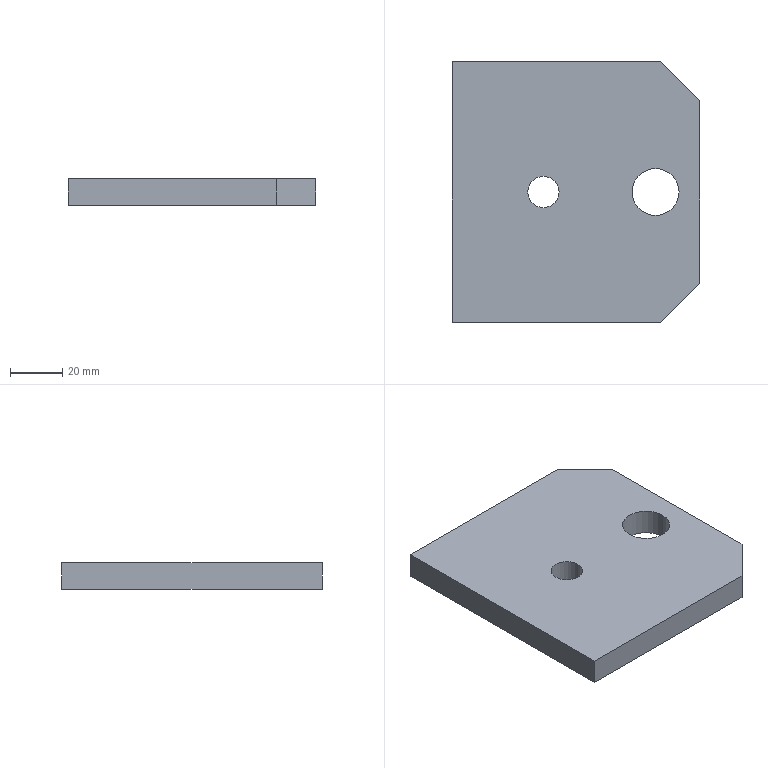Part | SolidWorks | features Extrusion 1 | 1 solid | 12 faces | box 95 x 100 x 10 mm | volume 89074 mm3 | plane 8 | cylinder 4 | commonest cylinder face diameters 12 x2 18 x2
STEP:
#1=CARTESIAN_POINT('',(21.5,0.,10.));
#2=VERTEX_POINT('',#1);
#3=CARTESIAN_POINT('',(39.5,0.,10.));
#4=VERTEX_POINT('',#3);
#5=CARTESIAN_POINT('',(30.5,0.,10.));
#6=DIRECTION('',(0.,0.,1.));
#7=DIRECTION('',(1.,0.,0.));
#8=AXIS2_PLACEMENT_3D('',#5,#6,#7);
#9=CIRCLE('',#8,9.);
#10=EDGE_CURVE('',#2,#4,#9,.T.);
#11=ORIENTED_EDGE('',*,*,#10,.T.);
#12=CARTESIAN_POINT('',(39.5,0.,0.));
#13=VERTEX_POINT('',#12);
#14=CARTESIAN_POINT('',(39.5,0.,10.));
#15=DIRECTION('',(0.,0.,-1.));
#16=VECTOR('',#15,1000.);
#17=LINE('',#14,#16);
#18=EDGE_CURVE('',#4,#13,#17,.T.);
#19=ORIENTED_EDGE('',*,*,#18,.T.);
#20=CARTESIAN_POINT('',(21.5,0.,0.));
#21=VERTEX_POINT('',#20);
#22=CARTESIAN_POINT('',(30.5,0.,0.));
#23=DIRECTION('',(0.,0.,1.));
#24=DIRECTION('',(1.,0.,0.));
#25=AXIS2_PLACEMENT_3D('',#22,#23,#24);
#26=CIRCLE('',#25,9.);
#27=EDGE_CURVE('',#21,#13,#26,.T.);
#28=ORIENTED_EDGE('',*,*,#27,.F.);
#29=CARTESIAN_POINT('',(21.5,0.,10.));
#30=DIRECTION('',(0.,0.,-1.));
#31=VECTOR('',#30,1000.);
#32=LINE('',#29,#31);
#33=EDGE_CURVE('',#2,#21,#32,.T.);
#34=ORIENTED_EDGE('',*,*,#33,.F.);
#35=EDGE_LOOP('',(#11,#19,#28,#34));
#36=FACE_OUTER_BOUND('',#35,.T.);
#37=CARTESIAN_POINT('',(30.5,0.,10.));
#38=DIRECTION('',(0.,0.,-1.));
#39=DIRECTION('',(-1.,0.,0.));
#40=AXIS2_PLACEMENT_3D('',#37,#38,#39);
#41=CYLINDRICAL_SURFACE('',#40,9.);
#42=ADVANCED_FACE('',(#36),#41,.F.);
#43=CARTESIAN_POINT('',(-18.5,0.,10.));
#44=VERTEX_POINT('',#43);
#45=CARTESIAN_POINT('',(-6.5,0.,10.));
#46=VERTEX_POINT('',#45);
#47=CARTESIAN_POINT('',(-12.5,0.,10.));
#48=DIRECTION('',(0.,0.,1.));
#49=DIRECTION('',(1.,0.,0.));
#50=AXIS2_PLACEMENT_3D('',#47,#48,#49);
#51=CIRCLE('',#50,6.);
#52=EDGE_CURVE('',#44,#46,#51,.T.);
#53=ORIENTED_EDGE('',*,*,#52,.T.);
#54=CARTESIAN_POINT('',(-6.5,0.,0.));
#55=VERTEX_POINT('',#54);
#56=CARTESIAN_POINT('',(-6.5,0.,10.));
#57=DIRECTION('',(0.,0.,-1.));
#58=VECTOR('',#57,1000.);
#59=LINE('',#56,#58);
#60=EDGE_CURVE('',#46,#55,#59,.T.);
#61=ORIENTED_EDGE('',*,*,#60,.T.);
#62=CARTESIAN_POINT('',(-18.5,0.,0.));
#63=VERTEX_POINT('',#62);
#64=CARTESIAN_POINT('',(-12.5,0.,0.));
#65=DIRECTION('',(0.,0.,1.));
#66=DIRECTION('',(1.,0.,0.));
#67=AXIS2_PLACEMENT_3D('',#64,#65,#66);
#68=CIRCLE('',#67,6.);
#69=EDGE_CURVE('',#63,#55,#68,.T.);
#70=ORIENTED_EDGE('',*,*,#69,.F.);
#71=CARTESIAN_POINT('',(-18.5,0.,10.));
#72=DIRECTION('',(0.,0.,-1.));
#73=VECTOR('',#72,1000.);
#74=LINE('',#71,#73);
#75=EDGE_CURVE('',#44,#63,#74,.T.);
#76=ORIENTED_EDGE('',*,*,#75,.F.);
#77=EDGE_LOOP('',(#53,#61,#70,#76));
#78=FACE_OUTER_BOUND('',#77,.T.);
#79=CARTESIAN_POINT('',(-12.5,0.,10.));
#80=DIRECTION('',(0.,0.,-1.));
#81=DIRECTION('',(-1.,0.,0.));
#82=AXIS2_PLACEMENT_3D('',#79,#80,#81);
#83=CYLINDRICAL_SURFACE('',#82,6.);
#84=ADVANCED_FACE('',(#78),#83,.F.);
#85=CARTESIAN_POINT('',(-47.5,50.,10.));
#86=VERTEX_POINT('',#85);
#87=CARTESIAN_POINT('',(-47.5,-50.,10.));
#88=VERTEX_POINT('',#87);
#89=CARTESIAN_POINT('',(-47.5,50.,10.));
#90=DIRECTION('',(0.,-1.,0.));
#91=VECTOR('',#90,1000.);
#92=LINE('',#89,#91);
#93=EDGE_CURVE('',#86,#88,#92,.T.);
#94=ORIENTED_EDGE('',*,*,#93,.T.);
#95=CARTESIAN_POINT('',(32.5,-50.,10.));
#96=VERTEX_POINT('',#95);
#97=CARTESIAN_POINT('',(32.5,-50.,10.));
#98=DIRECTION('',(1.,0.,0.));
#99=VECTOR('',#98,1000.);
#100=LINE('',#97,#99);
#101=EDGE_CURVE('',#88,#96,#100,.T.);
#102=ORIENTED_EDGE('',*,*,#101,.T.);
#103=CARTESIAN_POINT('',(47.5,-35.,10.));
#104=VERTEX_POINT('',#103);
#105=CARTESIAN_POINT('',(47.5,-35.,10.));
#106=DIRECTION('',(0.7071,0.7071,0.));
#107=VECTOR('',#106,1000.);
#108=LINE('',#105,#107);
#109=EDGE_CURVE('',#96,#104,#108,.T.);
#110=ORIENTED_EDGE('',*,*,#109,.T.);
#111=CARTESIAN_POINT('',(47.5,35.,10.));
#112=VERTEX_POINT('',#111);
#113=CARTESIAN_POINT('',(47.5,35.,10.));
#114=DIRECTION('',(0.,1.,0.));
#115=VECTOR('',#114,1000.);
#116=LINE('',#113,#115);
#117=EDGE_CURVE('',#104,#112,#116,.T.);
#118=ORIENTED_EDGE('',*,*,#117,.T.);
#119=CARTESIAN_POINT('',(32.5,50.,10.));
#120=VERTEX_POINT('',#119);
#121=CARTESIAN_POINT('',(47.5,35.,10.));
#122=DIRECTION('',(-0.7071,0.7071,0.));
#123=VECTOR('',#122,1000.);
#124=LINE('',#121,#123);
#125=EDGE_CURVE('',#112,#120,#124,.T.);
#126=ORIENTED_EDGE('',*,*,#125,.T.);
#127=CARTESIAN_POINT('',(32.5,50.,10.));
#128=DIRECTION('',(-1.,0.,0.));
#129=VECTOR('',#128,1000.);
#130=LINE('',#127,#129);
#131=EDGE_CURVE('',#120,#86,#130,.T.);
#132=ORIENTED_EDGE('',*,*,#131,.T.);
#133=EDGE_LOOP('',(#94,#102,#110,#118,#126,#132));
#134=FACE_OUTER_BOUND('',#133,.T.);
#135=ORIENTED_EDGE('',*,*,#52,.F.);
#136=CARTESIAN_POINT('',(-12.5,0.,10.));
#137=DIRECTION('',(0.,0.,1.));
#138=DIRECTION('',(1.,0.,0.));
#139=AXIS2_PLACEMENT_3D('',#136,#137,#138);
#140=CIRCLE('',#139,6.);
#141=EDGE_CURVE('',#46,#44,#140,.T.);
#142=ORIENTED_EDGE('',*,*,#141,.F.);
#143=EDGE_LOOP('',(#135,#142));
#144=FACE_BOUND('',#143,.T.);
#145=ORIENTED_EDGE('',*,*,#10,.F.);
#146=CARTESIAN_POINT('',(30.5,0.,10.));
#147=DIRECTION('',(0.,0.,1.));
#148=DIRECTION('',(1.,0.,0.));
#149=AXIS2_PLACEMENT_3D('',#146,#147,#148);
#150=CIRCLE('',#149,9.);
#151=EDGE_CURVE('',#4,#2,#150,.T.);
#152=ORIENTED_EDGE('',*,*,#151,.F.);
#153=EDGE_LOOP('',(#145,#152));
#154=FACE_BOUND('',#153,.T.);
#155=CARTESIAN_POINT('',(0.,0.,10.));
#156=DIRECTION('',(0.,0.,-1.));
#157=DIRECTION('',(-1.,0.,0.));
#158=AXIS2_PLACEMENT_3D('',#155,#156,#157);
#159=PLANE('',#158);
#160=ADVANCED_FACE('',(#134,#144,#154),#159,.F.);
#161=ORIENTED_EDGE('',*,*,#69,.T.);
#162=CARTESIAN_POINT('',(-12.5,0.,0.));
#163=DIRECTION('',(0.,0.,1.));
#164=DIRECTION('',(1.,0.,0.));
#165=AXIS2_PLACEMENT_3D('',#162,#163,#164);
#166=CIRCLE('',#165,6.);
#167=EDGE_CURVE('',#55,#63,#166,.T.);
#168=ORIENTED_EDGE('',*,*,#167,.T.);
#169=EDGE_LOOP('',(#161,#168));
#170=FACE_BOUND('',#169,.T.);
#171=CARTESIAN_POINT('',(-47.5,50.,0.));
#172=VERTEX_POINT('',#171);
#173=CARTESIAN_POINT('',(-47.5,-50.,0.));
#174=VERTEX_POINT('',#173);
#175=CARTESIAN_POINT('',(-47.5,50.,0.));
#176=DIRECTION('',(0.,-1.,0.));
#177=VECTOR('',#176,1000.);
#178=LINE('',#175,#177);
#179=EDGE_CURVE('',#172,#174,#178,.T.);
#180=ORIENTED_EDGE('',*,*,#179,.F.);
#181=CARTESIAN_POINT('',(32.5,50.,0.));
#182=VERTEX_POINT('',#181);
#183=CARTESIAN_POINT('',(32.5,50.,0.));
#184=DIRECTION('',(-1.,0.,0.));
#185=VECTOR('',#184,1000.);
#186=LINE('',#183,#185);
#187=EDGE_CURVE('',#182,#172,#186,.T.);
#188=ORIENTED_EDGE('',*,*,#187,.F.);
#189=CARTESIAN_POINT('',(47.5,35.,0.));
#190=VERTEX_POINT('',#189);
#191=CARTESIAN_POINT('',(47.5,35.,0.));
#192=DIRECTION('',(-0.7071,0.7071,0.));
#193=VECTOR('',#192,1000.);
#194=LINE('',#191,#193);
#195=EDGE_CURVE('',#190,#182,#194,.T.);
#196=ORIENTED_EDGE('',*,*,#195,.F.);
#197=CARTESIAN_POINT('',(47.5,-35.,0.));
#198=VERTEX_POINT('',#197);
#199=CARTESIAN_POINT('',(47.5,35.,0.));
#200=DIRECTION('',(0.,1.,0.));
#201=VECTOR('',#200,1000.);
#202=LINE('',#199,#201);
#203=EDGE_CURVE('',#198,#190,#202,.T.);
#204=ORIENTED_EDGE('',*,*,#203,.F.);
#205=CARTESIAN_POINT('',(32.5,-50.,0.));
#206=VERTEX_POINT('',#205);
#207=CARTESIAN_POINT('',(47.5,-35.,0.));
#208=DIRECTION('',(0.7071,0.7071,0.));
#209=VECTOR('',#208,1000.);
#210=LINE('',#207,#209);
#211=EDGE_CURVE('',#206,#198,#210,.T.);
#212=ORIENTED_EDGE('',*,*,#211,.F.);
#213=CARTESIAN_POINT('',(32.5,-50.,0.));
#214=DIRECTION('',(1.,0.,0.));
#215=VECTOR('',#214,1000.);
#216=LINE('',#213,#215);
#217=EDGE_CURVE('',#174,#206,#216,.T.);
#218=ORIENTED_EDGE('',*,*,#217,.F.);
#219=EDGE_LOOP('',(#180,#188,#196,#204,#212,#218));
#220=FACE_OUTER_BOUND('',#219,.T.);
#221=ORIENTED_EDGE('',*,*,#27,.T.);
#222=CARTESIAN_POINT('',(30.5,0.,0.));
#223=DIRECTION('',(0.,0.,1.));
#224=DIRECTION('',(1.,0.,0.));
#225=AXIS2_PLACEMENT_3D('',#222,#223,#224);
#226=CIRCLE('',#225,9.);
#227=EDGE_CURVE('',#13,#21,#226,.T.);
#228=ORIENTED_EDGE('',*,*,#227,.T.);
#229=EDGE_LOOP('',(#221,#228));
#230=FACE_BOUND('',#229,.T.);
#231=CARTESIAN_POINT('',(0.,0.,0.));
#232=DIRECTION('',(0.,0.,-1.));
#233=DIRECTION('',(-1.,0.,0.));
#234=AXIS2_PLACEMENT_3D('',#231,#232,#233);
#235=PLANE('',#234);
#236=ADVANCED_FACE('',(#170,#220,#230),#235,.T.);
#237=ORIENTED_EDGE('',*,*,#179,.T.);
#238=CARTESIAN_POINT('',(-47.5,-50.,10.));
#239=DIRECTION('',(0.,0.,-1.));
#240=VECTOR('',#239,1000.);
#241=LINE('',#238,#240);
#242=EDGE_CURVE('',#88,#174,#241,.T.);
#243=ORIENTED_EDGE('',*,*,#242,.F.);
#244=ORIENTED_EDGE('',*,*,#93,.F.);
#245=CARTESIAN_POINT('',(-47.5,50.,10.));
#246=DIRECTION('',(0.,0.,-1.));
#247=VECTOR('',#246,1000.);
#248=LINE('',#245,#247);
#249=EDGE_CURVE('',#86,#172,#248,.T.);
#250=ORIENTED_EDGE('',*,*,#249,.T.);
#251=EDGE_LOOP('',(#237,#243,#244,#250));
#252=FACE_OUTER_BOUND('',#251,.T.);
#253=CARTESIAN_POINT('',(-47.5,50.,10.));
#254=DIRECTION('',(1.,0.,0.));
#255=DIRECTION('',(0.,1.,0.));
#256=AXIS2_PLACEMENT_3D('',#253,#254,#255);
#257=PLANE('',#256);
#258=ADVANCED_FACE('',(#252),#257,.F.);
#259=ORIENTED_EDGE('',*,*,#217,.T.);
#260=CARTESIAN_POINT('',(32.5,-50.,10.));
#261=DIRECTION('',(0.,0.,-1.));
#262=VECTOR('',#261,1000.);
#263=LINE('',#260,#262);
#264=EDGE_CURVE('',#96,#206,#263,.T.);
#265=ORIENTED_EDGE('',*,*,#264,.F.);
#266=ORIENTED_EDGE('',*,*,#101,.F.);
#267=ORIENTED_EDGE('',*,*,#242,.T.);
#268=EDGE_LOOP('',(#259,#265,#266,#267));
#269=FACE_OUTER_BOUND('',#268,.T.);
#270=CARTESIAN_POINT('',(32.5,-50.,10.));
#271=DIRECTION('',(0.,1.,0.));
#272=DIRECTION('',(-1.,0.,0.));
#273=AXIS2_PLACEMENT_3D('',#270,#271,#272);
#274=PLANE('',#273);
#275=ADVANCED_FACE('',(#269),#274,.F.);
#276=ORIENTED_EDGE('',*,*,#211,.T.);
#277=CARTESIAN_POINT('',(47.5,-35.,10.));
#278=DIRECTION('',(0.,0.,-1.));
#279=VECTOR('',#278,1000.);
#280=LINE('',#277,#279);
#281=EDGE_CURVE('',#104,#198,#280,.T.);
#282=ORIENTED_EDGE('',*,*,#281,.F.);
#283=ORIENTED_EDGE('',*,*,#109,.F.);
#284=ORIENTED_EDGE('',*,*,#264,.T.);
#285=EDGE_LOOP('',(#276,#282,#283,#284));
#286=FACE_OUTER_BOUND('',#285,.T.);
#287=CARTESIAN_POINT('',(47.5,-35.,10.));
#288=DIRECTION('',(-0.7071,0.7071,0.));
#289=DIRECTION('',(-0.7071,-0.7071,0.));
#290=AXIS2_PLACEMENT_3D('',#287,#288,#289);
#291=PLANE('',#290);
#292=ADVANCED_FACE('',(#286),#291,.F.);
#293=ORIENTED_EDGE('',*,*,#203,.T.);
#294=CARTESIAN_POINT('',(47.5,35.,10.));
#295=DIRECTION('',(0.,0.,-1.));
#296=VECTOR('',#295,1000.);
#297=LINE('',#294,#296);
#298=EDGE_CURVE('',#112,#190,#297,.T.);
#299=ORIENTED_EDGE('',*,*,#298,.F.);
#300=ORIENTED_EDGE('',*,*,#117,.F.);
#301=ORIENTED_EDGE('',*,*,#281,.T.);
#302=EDGE_LOOP('',(#293,#299,#300,#301));
#303=FACE_OUTER_BOUND('',#302,.T.);
#304=CARTESIAN_POINT('',(47.5,35.,10.));
#305=DIRECTION('',(-1.,0.,0.));
#306=DIRECTION('',(0.,-1.,0.));
#307=AXIS2_PLACEMENT_3D('',#304,#305,#306);
#308=PLANE('',#307);
#309=ADVANCED_FACE('',(#303),#308,.F.);
#310=ORIENTED_EDGE('',*,*,#195,.T.);
#311=CARTESIAN_POINT('',(32.5,50.,10.));
#312=DIRECTION('',(0.,0.,-1.));
#313=VECTOR('',#312,1000.);
#314=LINE('',#311,#313);
#315=EDGE_CURVE('',#120,#182,#314,.T.);
#316=ORIENTED_EDGE('',*,*,#315,.F.);
#317=ORIENTED_EDGE('',*,*,#125,.F.);
#318=ORIENTED_EDGE('',*,*,#298,.T.);
#319=EDGE_LOOP('',(#310,#316,#317,#318));
#320=FACE_OUTER_BOUND('',#319,.T.);
#321=CARTESIAN_POINT('',(47.5,35.,10.));
#322=DIRECTION('',(-0.7071,-0.7071,0.));
#323=DIRECTION('',(0.7071,-0.7071,0.));
#324=AXIS2_PLACEMENT_3D('',#321,#322,#323);
#325=PLANE('',#324);
#326=ADVANCED_FACE('',(#320),#325,.F.);
#327=ORIENTED_EDGE('',*,*,#187,.T.);
#328=ORIENTED_EDGE('',*,*,#249,.F.);
#329=ORIENTED_EDGE('',*,*,#131,.F.);
#330=ORIENTED_EDGE('',*,*,#315,.T.);
#331=EDGE_LOOP('',(#327,#328,#329,#330));
#332=FACE_OUTER_BOUND('',#331,.T.);
#333=CARTESIAN_POINT('',(32.5,50.,10.));
#334=DIRECTION('',(0.,-1.,0.));
#335=DIRECTION('',(1.,0.,0.));
#336=AXIS2_PLACEMENT_3D('',#333,#334,#335);
#337=PLANE('',#336);
#338=ADVANCED_FACE('',(#332),#337,.F.);
#339=ORIENTED_EDGE('',*,*,#60,.F.);
#340=ORIENTED_EDGE('',*,*,#141,.T.);
#341=ORIENTED_EDGE('',*,*,#75,.T.);
#342=ORIENTED_EDGE('',*,*,#167,.F.);
#343=EDGE_LOOP('',(#339,#340,#341,#342));
#344=FACE_OUTER_BOUND('',#343,.T.);
#345=CARTESIAN_POINT('',(-12.5,0.,10.));
#346=DIRECTION('',(0.,0.,-1.));
#347=DIRECTION('',(-1.,0.,0.));
#348=AXIS2_PLACEMENT_3D('',#345,#346,#347);
#349=CYLINDRICAL_SURFACE('',#348,6.);
#350=ADVANCED_FACE('',(#344),#349,.F.);
#351=ORIENTED_EDGE('',*,*,#18,.F.);
#352=ORIENTED_EDGE('',*,*,#151,.T.);
#353=ORIENTED_EDGE('',*,*,#33,.T.);
#354=ORIENTED_EDGE('',*,*,#227,.F.);
#355=EDGE_LOOP('',(#351,#352,#353,#354));
#356=FACE_OUTER_BOUND('',#355,.T.);
#357=CARTESIAN_POINT('',(30.5,0.,10.));
#358=DIRECTION('',(0.,0.,-1.));
#359=DIRECTION('',(-1.,0.,0.));
#360=AXIS2_PLACEMENT_3D('',#357,#358,#359);
#361=CYLINDRICAL_SURFACE('',#360,9.);
#362=ADVANCED_FACE('',(#356),#361,.F.);
#363=CLOSED_SHELL('',(#42,#84,#160,#236,#258,#275,#292,#309,#326,#338,#350,#362));
#364=MANIFOLD_SOLID_BREP('',#363);
#365=CARTESIAN_POINT('',(0.,0.,0.));
#366=DIRECTION('',(0.,0.,1.));
#367=DIRECTION('',(1.,0.,0.));
#368=AXIS2_PLACEMENT_3D('',#365,#366,#367);
#369=(LENGTH_UNIT()NAMED_UNIT(*)SI_UNIT(.MILLI.,.METRE.));
#370=UNCERTAINTY_MEASURE_WITH_UNIT(LENGTH_MEASURE(0.00001),#369,'','');
#371=(NAMED_UNIT(*)PLANE_ANGLE_UNIT()SI_UNIT($,.RADIAN.));
#372=(NAMED_UNIT(*)SI_UNIT($,.STERADIAN.)SOLID_ANGLE_UNIT());
#373=(GEOMETRIC_REPRESENTATION_CONTEXT(3)GLOBAL_UNCERTAINTY_ASSIGNED_CONTEXT((#370))GLOBAL_UNIT_ASSIGNED_CONTEXT((#369,#371,#372))REPRESENTATION_CONTEXT('',''));
#374=ADVANCED_BREP_SHAPE_REPRESENTATION('',(#364,#368),#373);